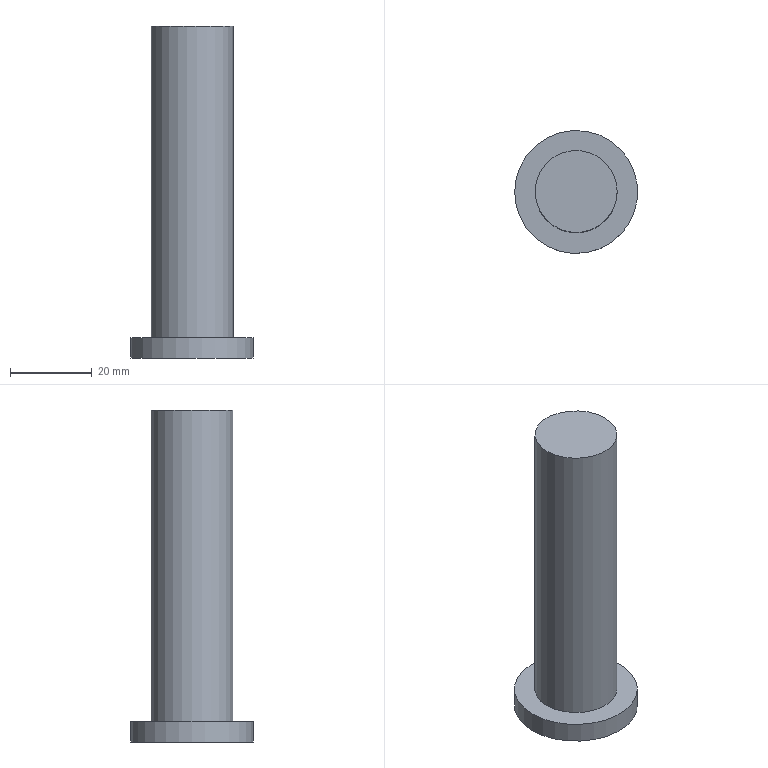Part | NX | features 脚踏板柱销 2 | 1 solid | 5 faces | box 30 x 30 x 81 mm | volume 27410 mm3 | plane 3 | cylinder 2 | commonest cylinder face diameters 20 x1 30 x1
STEP:
#1=CARTESIAN_POINT('',(10.,0.,76.));
#2=VERTEX_POINT('',#1);
#3=CARTESIAN_POINT('',(0.,0.,76.));
#4=DIRECTION('',(0.,0.,1.));
#5=DIRECTION('',(1.,0.,0.));
#6=AXIS2_PLACEMENT_3D('',#3,#4,#5);
#7=CIRCLE('',#6,10.);
#8=EDGE_CURVE('',#2,#2,#7,.T.);
#9=ORIENTED_EDGE('',*,*,#8,.F.);
#10=EDGE_LOOP('',(#9));
#11=FACE_BOUND('',#10,.T.);
#12=CARTESIAN_POINT('',(-10.,0.,0.));
#13=VERTEX_POINT('',#12);
#14=CARTESIAN_POINT('',(0.,0.,0.));
#15=DIRECTION('',(0.,0.,-1.));
#16=DIRECTION('',(-1.,0.,0.));
#17=AXIS2_PLACEMENT_3D('',#14,#15,#16);
#18=CIRCLE('',#17,10.);
#19=EDGE_CURVE('',#13,#13,#18,.T.);
#20=ORIENTED_EDGE('',*,*,#19,.F.);
#21=EDGE_LOOP('',(#20));
#22=FACE_BOUND('',#21,.T.);
#23=CARTESIAN_POINT('',(0.,0.,76.));
#24=DIRECTION('',(0.,0.,-1.));
#25=DIRECTION('',(-1.,0.,0.));
#26=AXIS2_PLACEMENT_3D('',#23,#24,#25);
#27=CYLINDRICAL_SURFACE('',#26,10.);
#28=ADVANCED_FACE('',(#11,#22),#27,.T.);
#29=ORIENTED_EDGE('',*,*,#8,.T.);
#30=EDGE_LOOP('',(#29));
#31=FACE_BOUND('',#30,.T.);
#32=CARTESIAN_POINT('',(0.,0.,76.));
#33=DIRECTION('',(0.,0.,1.));
#34=DIRECTION('',(1.,0.,0.));
#35=AXIS2_PLACEMENT_3D('',#32,#33,#34);
#36=PLANE('',#35);
#37=ADVANCED_FACE('',(#31),#36,.T.);
#38=CARTESIAN_POINT('',(-15.,0.,0.));
#39=VERTEX_POINT('',#38);
#40=CARTESIAN_POINT('',(0.,0.,0.));
#41=DIRECTION('',(0.,0.,-1.));
#42=DIRECTION('',(-1.,0.,0.));
#43=AXIS2_PLACEMENT_3D('',#40,#41,#42);
#44=CIRCLE('',#43,15.);
#45=EDGE_CURVE('',#39,#39,#44,.T.);
#46=ORIENTED_EDGE('',*,*,#45,.F.);
#47=EDGE_LOOP('',(#46));
#48=FACE_BOUND('',#47,.T.);
#49=ORIENTED_EDGE('',*,*,#19,.T.);
#50=EDGE_LOOP('',(#49));
#51=FACE_BOUND('',#50,.T.);
#52=CARTESIAN_POINT('',(0.,0.,0.));
#53=DIRECTION('',(0.,0.,-1.));
#54=DIRECTION('',(-1.,0.,0.));
#55=AXIS2_PLACEMENT_3D('',#52,#53,#54);
#56=PLANE('',#55);
#57=ADVANCED_FACE('',(#48,#51),#56,.F.);
#58=CARTESIAN_POINT('',(-15.,0.,-5.));
#59=VERTEX_POINT('',#58);
#60=CARTESIAN_POINT('',(0.,0.,-5.));
#61=DIRECTION('',(0.,0.,-1.));
#62=DIRECTION('',(-1.,0.,0.));
#63=AXIS2_PLACEMENT_3D('',#60,#61,#62);
#64=CIRCLE('',#63,15.);
#65=EDGE_CURVE('',#59,#59,#64,.T.);
#66=ORIENTED_EDGE('',*,*,#65,.F.);
#67=EDGE_LOOP('',(#66));
#68=FACE_BOUND('',#67,.T.);
#69=ORIENTED_EDGE('',*,*,#45,.T.);
#70=EDGE_LOOP('',(#69));
#71=FACE_BOUND('',#70,.T.);
#72=CARTESIAN_POINT('',(0.,0.,-5.));
#73=DIRECTION('',(0.,0.,1.));
#74=DIRECTION('',(1.,0.,0.));
#75=AXIS2_PLACEMENT_3D('',#72,#73,#74);
#76=CYLINDRICAL_SURFACE('',#75,15.);
#77=ADVANCED_FACE('',(#68,#71),#76,.T.);
#78=ORIENTED_EDGE('',*,*,#65,.T.);
#79=EDGE_LOOP('',(#78));
#80=FACE_BOUND('',#79,.T.);
#81=CARTESIAN_POINT('',(0.,0.,-5.));
#82=DIRECTION('',(0.,0.,-1.));
#83=DIRECTION('',(-1.,0.,0.));
#84=AXIS2_PLACEMENT_3D('',#81,#82,#83);
#85=PLANE('',#84);
#86=ADVANCED_FACE('',(#80),#85,.T.);
#87=CLOSED_SHELL('',(#28,#37,#57,#77,#86));
#88=MANIFOLD_SOLID_BREP('',#87);
#89=(LENGTH_UNIT()NAMED_UNIT(*)SI_UNIT(.MILLI.,.METRE.));
#90=UNCERTAINTY_MEASURE_WITH_UNIT(LENGTH_MEASURE(0.00001),#89,'','');
#91=(NAMED_UNIT(*)PLANE_ANGLE_UNIT()SI_UNIT($,.RADIAN.));
#92=(NAMED_UNIT(*)SI_UNIT($,.STERADIAN.)SOLID_ANGLE_UNIT());
#93=(GEOMETRIC_REPRESENTATION_CONTEXT(3)GLOBAL_UNCERTAINTY_ASSIGNED_CONTEXT((#90))GLOBAL_UNIT_ASSIGNED_CONTEXT((#89,#91,#92))REPRESENTATION_CONTEXT('',''));
#94=ADVANCED_BREP_SHAPE_REPRESENTATION('',(#88),#93);